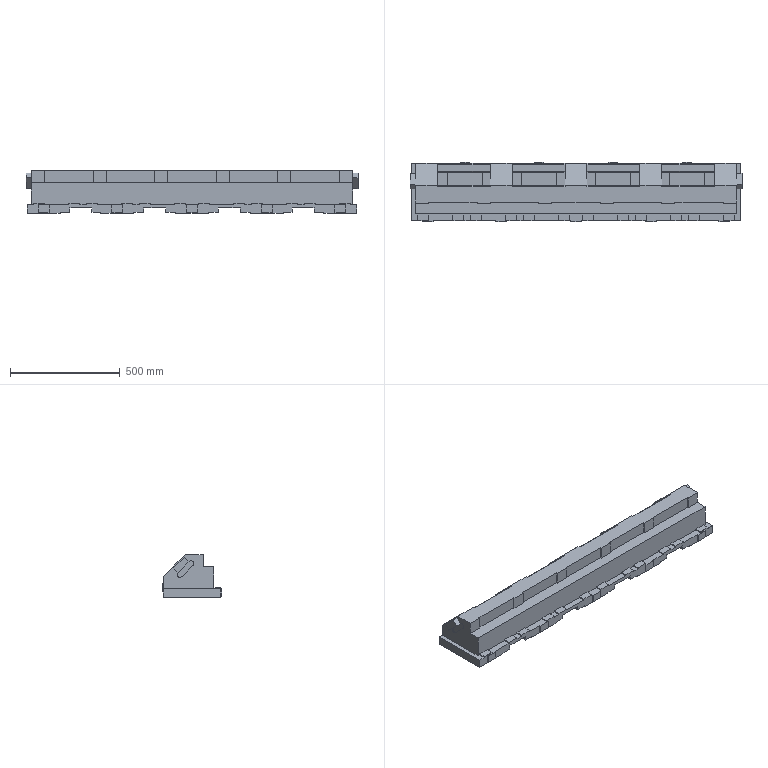Part | NX | features solid 2 | 1 solid | 279 faces | box 1510 x 270 x 195 mm | volume 40094196 mm3 | plane 259 | cylinder 20 | commonest cylinder face diameters 10 x16 25 x4